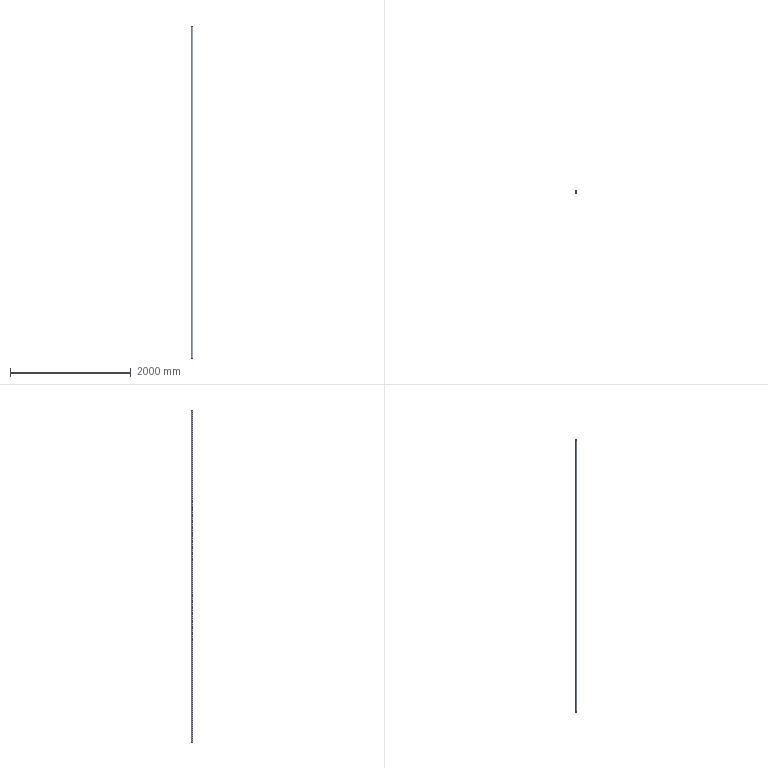Part | SolidWorks | features Extrusion 1 | 1 solid | 4 faces | box 30 x 30 x 5500 mm | volume 3887721 mm3 | cylinder 2 | plane 2 | commonest cylinder face diameters 30 x2
STEP:
#1=CARTESIAN_POINT('',(15.,0.,5500.));
#2=VERTEX_POINT('',#1);
#3=CARTESIAN_POINT('',(-15.,0.,5500.));
#4=VERTEX_POINT('',#3);
#5=CARTESIAN_POINT('',(0.,0.,5500.));
#6=DIRECTION('',(0.,0.,1.));
#7=DIRECTION('',(1.,0.,0.));
#8=AXIS2_PLACEMENT_3D('',#5,#6,#7);
#9=CIRCLE('',#8,15.);
#10=EDGE_CURVE('',#2,#4,#9,.T.);
#11=ORIENTED_EDGE('',*,*,#10,.F.);
#12=CARTESIAN_POINT('',(15.,0.,0.));
#13=VERTEX_POINT('',#12);
#14=CARTESIAN_POINT('',(15.,0.,5500.));
#15=DIRECTION('',(0.,0.,-1.));
#16=VECTOR('',#15,1000.);
#17=LINE('',#14,#16);
#18=EDGE_CURVE('',#2,#13,#17,.T.);
#19=ORIENTED_EDGE('',*,*,#18,.T.);
#20=CARTESIAN_POINT('',(-15.,0.,0.));
#21=VERTEX_POINT('',#20);
#22=CARTESIAN_POINT('',(0.,0.,0.));
#23=DIRECTION('',(0.,0.,1.));
#24=DIRECTION('',(1.,0.,0.));
#25=AXIS2_PLACEMENT_3D('',#22,#23,#24);
#26=CIRCLE('',#25,15.);
#27=EDGE_CURVE('',#13,#21,#26,.T.);
#28=ORIENTED_EDGE('',*,*,#27,.T.);
#29=CARTESIAN_POINT('',(-15.,0.,5500.));
#30=DIRECTION('',(0.,0.,-1.));
#31=VECTOR('',#30,1000.);
#32=LINE('',#29,#31);
#33=EDGE_CURVE('',#4,#21,#32,.T.);
#34=ORIENTED_EDGE('',*,*,#33,.F.);
#35=EDGE_LOOP('',(#11,#19,#28,#34));
#36=FACE_OUTER_BOUND('',#35,.T.);
#37=CARTESIAN_POINT('',(0.,0.,5500.));
#38=DIRECTION('',(0.,0.,-1.));
#39=DIRECTION('',(-1.,0.,0.));
#40=AXIS2_PLACEMENT_3D('',#37,#38,#39);
#41=CYLINDRICAL_SURFACE('',#40,15.);
#42=ADVANCED_FACE('',(#36),#41,.T.);
#43=ORIENTED_EDGE('',*,*,#18,.F.);
#44=CARTESIAN_POINT('',(0.,0.,5500.));
#45=DIRECTION('',(0.,0.,1.));
#46=DIRECTION('',(1.,0.,0.));
#47=AXIS2_PLACEMENT_3D('',#44,#45,#46);
#48=CIRCLE('',#47,15.);
#49=EDGE_CURVE('',#4,#2,#48,.T.);
#50=ORIENTED_EDGE('',*,*,#49,.F.);
#51=ORIENTED_EDGE('',*,*,#33,.T.);
#52=CARTESIAN_POINT('',(0.,0.,0.));
#53=DIRECTION('',(0.,0.,1.));
#54=DIRECTION('',(1.,0.,0.));
#55=AXIS2_PLACEMENT_3D('',#52,#53,#54);
#56=CIRCLE('',#55,15.);
#57=EDGE_CURVE('',#21,#13,#56,.T.);
#58=ORIENTED_EDGE('',*,*,#57,.T.);
#59=EDGE_LOOP('',(#43,#50,#51,#58));
#60=FACE_OUTER_BOUND('',#59,.T.);
#61=CARTESIAN_POINT('',(0.,0.,5500.));
#62=DIRECTION('',(0.,0.,-1.));
#63=DIRECTION('',(-1.,0.,0.));
#64=AXIS2_PLACEMENT_3D('',#61,#62,#63);
#65=CYLINDRICAL_SURFACE('',#64,15.);
#66=ADVANCED_FACE('',(#60),#65,.T.);
#67=ORIENTED_EDGE('',*,*,#49,.T.);
#68=ORIENTED_EDGE('',*,*,#10,.T.);
#69=EDGE_LOOP('',(#67,#68));
#70=FACE_OUTER_BOUND('',#69,.T.);
#71=CARTESIAN_POINT('',(0.,0.,5500.));
#72=DIRECTION('',(0.,0.,1.));
#73=DIRECTION('',(1.,0.,0.));
#74=AXIS2_PLACEMENT_3D('',#71,#72,#73);
#75=PLANE('',#74);
#76=ADVANCED_FACE('',(#70),#75,.T.);
#77=ORIENTED_EDGE('',*,*,#57,.F.);
#78=ORIENTED_EDGE('',*,*,#27,.F.);
#79=EDGE_LOOP('',(#77,#78));
#80=FACE_OUTER_BOUND('',#79,.T.);
#81=CARTESIAN_POINT('',(0.,0.,0.));
#82=DIRECTION('',(0.,0.,1.));
#83=DIRECTION('',(1.,0.,0.));
#84=AXIS2_PLACEMENT_3D('',#81,#82,#83);
#85=PLANE('',#84);
#86=ADVANCED_FACE('',(#80),#85,.F.);
#87=CLOSED_SHELL('',(#42,#66,#76,#86));
#88=MANIFOLD_SOLID_BREP('',#87);
#89=CARTESIAN_POINT('',(0.,0.,0.));
#90=DIRECTION('',(0.,0.,1.));
#91=DIRECTION('',(1.,0.,0.));
#92=AXIS2_PLACEMENT_3D('',#89,#90,#91);
#93=(LENGTH_UNIT()NAMED_UNIT(*)SI_UNIT(.MILLI.,.METRE.));
#94=UNCERTAINTY_MEASURE_WITH_UNIT(LENGTH_MEASURE(0.00001),#93,'','');
#95=(NAMED_UNIT(*)PLANE_ANGLE_UNIT()SI_UNIT($,.RADIAN.));
#96=(NAMED_UNIT(*)SI_UNIT($,.STERADIAN.)SOLID_ANGLE_UNIT());
#97=(GEOMETRIC_REPRESENTATION_CONTEXT(3)GLOBAL_UNCERTAINTY_ASSIGNED_CONTEXT((#94))GLOBAL_UNIT_ASSIGNED_CONTEXT((#93,#95,#96))REPRESENTATION_CONTEXT('',''));
#98=ADVANCED_BREP_SHAPE_REPRESENTATION('',(#88,#92),#97);